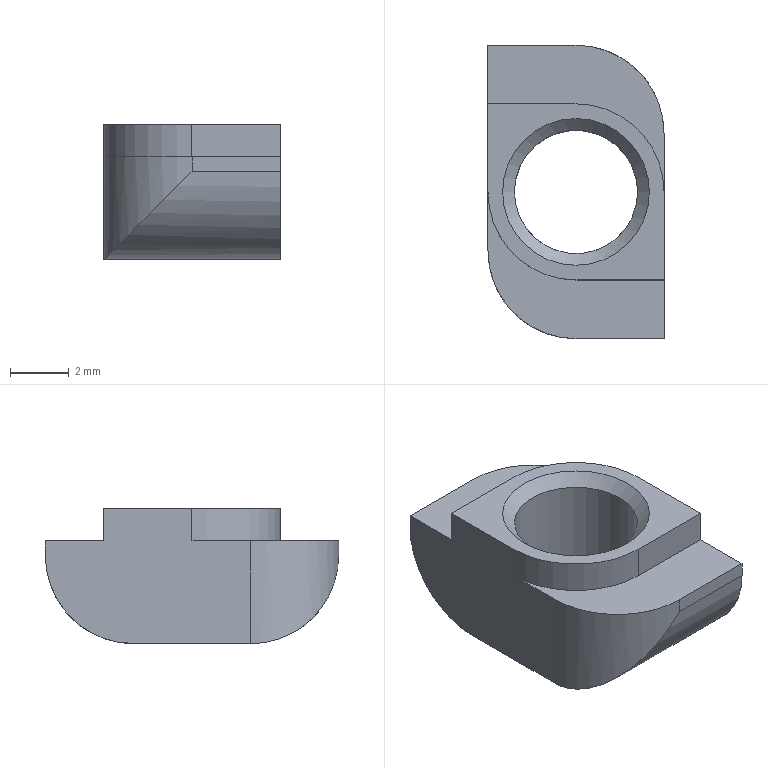Part | NX | features DATUM_CSYS 4, SKETCH 3, EXTRUDE 2, BLEND 1, HOLE PACKAGE 1, SIMPLE HOLE 1, SYMBOLIC_THREAD 1 | 1 solid | 19 faces | box 6 x 10 x 4.6 mm | volume 148.977 mm3 | plane 11 | cylinder 7 | cone 1 | commonest cylinder face diameters 6 x6 4.2 x1
STEP:
#1=CARTESIAN_POINT('',(3.,-2.,-3.5));
#2=VERTEX_POINT('',#1);
#3=CARTESIAN_POINT('',(0.6403,-2.,-3.5));
#4=VERTEX_POINT('',#3);
#5=CARTESIAN_POINT('',(3.,-2.,-3.5));
#6=DIRECTION('',(-1.,0.,0.));
#7=VECTOR('',#6,1000.);
#8=LINE('',#5,#7);
#9=EDGE_CURVE('',#2,#4,#8,.T.);
#10=ORIENTED_EDGE('',*,*,#9,.T.);
#11=CARTESIAN_POINT('',(0.6403,2.,-3.5));
#12=VERTEX_POINT('',#11);
#13=CARTESIAN_POINT('',(0.,0.,-3.5));
#14=DIRECTION('',(0.,0.,1.));
#15=DIRECTION('',(0.,-1.,0.));
#16=AXIS2_PLACEMENT_3D('',#13,#14,#15);
#17=CIRCLE('',#16,2.1);
#18=EDGE_CURVE('',#4,#12,#17,.T.);
#19=ORIENTED_EDGE('',*,*,#18,.T.);
#20=CARTESIAN_POINT('',(3.,2.,-3.5));
#21=VERTEX_POINT('',#20);
#22=CARTESIAN_POINT('',(3.,2.,-3.5));
#23=DIRECTION('',(-1.,0.,0.));
#24=VECTOR('',#23,1000.);
#25=LINE('',#22,#24);
#26=EDGE_CURVE('',#21,#12,#25,.T.);
#27=ORIENTED_EDGE('',*,*,#26,.F.);
#28=CARTESIAN_POINT('',(3.,-2.,-3.5));
#29=DIRECTION('',(0.,1.,0.));
#30=VECTOR('',#29,1000.);
#31=LINE('',#28,#30);
#32=EDGE_CURVE('',#2,#21,#31,.T.);
#33=ORIENTED_EDGE('',*,*,#32,.F.);
#34=EDGE_LOOP('',(#10,#19,#27,#33));
#35=FACE_BOUND('',#34,.T.);
#36=CARTESIAN_POINT('',(3.,0.,-3.5));
#37=DIRECTION('',(0.,0.,1.));
#38=DIRECTION('',(0.,-1.,0.));
#39=AXIS2_PLACEMENT_3D('',#36,#37,#38);
#40=PLANE('',#39);
#41=ADVANCED_FACE('',(#35),#40,.F.);
#42=CARTESIAN_POINT('',(0.,3.,0.));
#43=VERTEX_POINT('',#42);
#44=CARTESIAN_POINT('',(-3.,3.,0.));
#45=VERTEX_POINT('',#44);
#46=CARTESIAN_POINT('',(0.,3.,0.));
#47=DIRECTION('',(-1.,0.,0.));
#48=VECTOR('',#47,1000.);
#49=LINE('',#46,#48);
#50=EDGE_CURVE('',#43,#45,#49,.T.);
#51=ORIENTED_EDGE('',*,*,#50,.F.);
#52=CARTESIAN_POINT('',(3.,0.,0.));
#53=VERTEX_POINT('',#52);
#54=CARTESIAN_POINT('',(0.,0.,0.));
#55=DIRECTION('',(0.,0.,1.));
#56=DIRECTION('',(1.,0.,0.));
#57=AXIS2_PLACEMENT_3D('',#54,#55,#56);
#58=CIRCLE('',#57,3.);
#59=EDGE_CURVE('',#53,#43,#58,.T.);
#60=ORIENTED_EDGE('',*,*,#59,.F.);
#61=CARTESIAN_POINT('',(3.,2.,0.));
#62=VERTEX_POINT('',#61);
#63=CARTESIAN_POINT('',(3.,0.,0.));
#64=DIRECTION('',(0.,-1.,0.));
#65=VECTOR('',#64,1000.);
#66=LINE('',#63,#65);
#67=EDGE_CURVE('',#62,#53,#66,.T.);
#68=ORIENTED_EDGE('',*,*,#67,.F.);
#69=CARTESIAN_POINT('',(0.,5.,0.));
#70=VERTEX_POINT('',#69);
#71=CARTESIAN_POINT('',(0.,2.,0.));
#72=DIRECTION('',(0.,0.,-1.));
#73=DIRECTION('',(-1.,0.,0.));
#74=AXIS2_PLACEMENT_3D('',#71,#72,#73);
#75=CIRCLE('',#74,3.);
#76=EDGE_CURVE('',#62,#70,#75,.F.);
#77=ORIENTED_EDGE('',*,*,#76,.T.);
#78=CARTESIAN_POINT('',(-3.,5.,0.));
#79=VERTEX_POINT('',#78);
#80=CARTESIAN_POINT('',(3.,5.,0.));
#81=DIRECTION('',(-1.,0.,0.));
#82=VECTOR('',#81,1000.);
#83=LINE('',#80,#82);
#84=EDGE_CURVE('',#70,#79,#83,.T.);
#85=ORIENTED_EDGE('',*,*,#84,.T.);
#86=CARTESIAN_POINT('',(-3.,5.,0.));
#87=DIRECTION('',(0.,-1.,0.));
#88=VECTOR('',#87,1000.);
#89=LINE('',#86,#88);
#90=EDGE_CURVE('',#79,#45,#89,.T.);
#91=ORIENTED_EDGE('',*,*,#90,.T.);
#92=EDGE_LOOP('',(#51,#60,#68,#77,#85,#91));
#93=FACE_BOUND('',#92,.T.);
#94=CARTESIAN_POINT('',(3.,5.,0.));
#95=DIRECTION('',(0.,0.,-1.));
#96=DIRECTION('',(-1.,0.,0.));
#97=AXIS2_PLACEMENT_3D('',#94,#95,#96);
#98=PLANE('',#97);
#99=ADVANCED_FACE('',(#93),#98,.F.);
#100=CARTESIAN_POINT('',(3.,-5.,0.));
#101=VERTEX_POINT('',#100);
#102=CARTESIAN_POINT('',(0.,-5.,0.));
#103=VERTEX_POINT('',#102);
#104=CARTESIAN_POINT('',(3.,-5.,0.));
#105=DIRECTION('',(-1.,0.,0.));
#106=VECTOR('',#105,1000.);
#107=LINE('',#104,#106);
#108=EDGE_CURVE('',#101,#103,#107,.T.);
#109=ORIENTED_EDGE('',*,*,#108,.T.);
#110=CARTESIAN_POINT('',(0.,-5.,-0.5));
#111=VERTEX_POINT('',#110);
#112=CARTESIAN_POINT('',(0.,-5.,0.));
#113=DIRECTION('',(0.,0.,-1.));
#114=VECTOR('',#113,1000.);
#115=LINE('',#112,#114);
#116=EDGE_CURVE('',#103,#111,#115,.T.);
#117=ORIENTED_EDGE('',*,*,#116,.T.);
#118=CARTESIAN_POINT('',(3.,-5.,-0.5));
#119=VERTEX_POINT('',#118);
#120=CARTESIAN_POINT('',(3.,-5.,-0.5));
#121=DIRECTION('',(-1.,0.,0.));
#122=VECTOR('',#121,1000.);
#123=LINE('',#120,#122);
#124=EDGE_CURVE('',#119,#111,#123,.T.);
#125=ORIENTED_EDGE('',*,*,#124,.F.);
#126=CARTESIAN_POINT('',(3.,-5.,0.));
#127=DIRECTION('',(0.,0.,-1.));
#128=VECTOR('',#127,1000.);
#129=LINE('',#126,#128);
#130=EDGE_CURVE('',#101,#119,#129,.T.);
#131=ORIENTED_EDGE('',*,*,#130,.F.);
#132=EDGE_LOOP('',(#109,#117,#125,#131));
#133=FACE_BOUND('',#132,.T.);
#134=CARTESIAN_POINT('',(3.,-5.,0.));
#135=DIRECTION('',(0.,1.,0.));
#136=DIRECTION('',(0.,0.,1.));
#137=AXIS2_PLACEMENT_3D('',#134,#135,#136);
#138=PLANE('',#137);
#139=ADVANCED_FACE('',(#133),#138,.F.);
#140=CARTESIAN_POINT('',(-0.6403,-2.,-3.5));
#141=VERTEX_POINT('',#140);
#142=CARTESIAN_POINT('',(-3.,-2.,-3.5));
#143=VERTEX_POINT('',#142);
#144=CARTESIAN_POINT('',(3.,-2.,-3.5));
#145=DIRECTION('',(-1.,0.,0.));
#146=VECTOR('',#145,1000.);
#147=LINE('',#144,#146);
#148=EDGE_CURVE('',#141,#143,#147,.T.);
#149=ORIENTED_EDGE('',*,*,#148,.F.);
#150=CARTESIAN_POINT('',(-0.6403,-2.,-3.5));
#151=CARTESIAN_POINT('',(-0.2238,-2.133,-3.5));
#152=CARTESIAN_POINT('',(0.2238,-2.133,-3.5));
#153=CARTESIAN_POINT('',(0.6403,-2.,-3.5));
#154=B_SPLINE_CURVE_WITH_KNOTS('',3,(#150,#151,#152,#153),.UNSPECIFIED.,.F.,.F.,(4,4),(0.,0.001293),.UNSPECIFIED.);
#155=EDGE_CURVE('',#141,#4,#154,.T.);
#156=ORIENTED_EDGE('',*,*,#155,.T.);
#157=ORIENTED_EDGE('',*,*,#9,.F.);
#158=CARTESIAN_POINT('',(3.,-2.,-0.5));
#159=DIRECTION('',(1.,0.,0.));
#160=DIRECTION('',(0.,1.,0.));
#161=AXIS2_PLACEMENT_3D('',#158,#159,#160);
#162=CIRCLE('',#161,3.);
#163=EDGE_CURVE('',#119,#2,#162,.T.);
#164=ORIENTED_EDGE('',*,*,#163,.F.);
#165=ORIENTED_EDGE('',*,*,#124,.T.);
#166=CARTESIAN_POINT('',(0.,-2.,-0.5));
#167=DIRECTION('',(0.7071,0.,-0.7071));
#168=DIRECTION('',(-0.7071,0.,-0.7071));
#169=AXIS2_PLACEMENT_3D('',#166,#167,#168);
#170=ELLIPSE('',#169,4.243,3.);
#171=EDGE_CURVE('',#111,#143,#170,.T.);
#172=ORIENTED_EDGE('',*,*,#171,.T.);
#173=EDGE_LOOP('',(#149,#156,#157,#164,#165,#172));
#174=FACE_BOUND('',#173,.T.);
#175=CARTESIAN_POINT('',(3.,-2.,-0.5));
#176=DIRECTION('',(-1.,0.,0.));
#177=DIRECTION('',(0.,0.,1.));
#178=AXIS2_PLACEMENT_3D('',#175,#176,#177);
#179=CYLINDRICAL_SURFACE('',#178,3.);
#180=ADVANCED_FACE('',(#174),#179,.T.);
#181=CARTESIAN_POINT('',(-0.6403,2.,-3.5));
#182=VERTEX_POINT('',#181);
#183=CARTESIAN_POINT('',(-3.,2.,-3.5));
#184=VERTEX_POINT('',#183);
#185=CARTESIAN_POINT('',(3.,2.,-3.5));
#186=DIRECTION('',(-1.,0.,0.));
#187=VECTOR('',#186,1000.);
#188=LINE('',#185,#187);
#189=EDGE_CURVE('',#182,#184,#188,.T.);
#190=ORIENTED_EDGE('',*,*,#189,.F.);
#191=CARTESIAN_POINT('',(0.,0.,-3.5));
#192=DIRECTION('',(0.,0.,1.));
#193=DIRECTION('',(0.,-1.,0.));
#194=AXIS2_PLACEMENT_3D('',#191,#192,#193);
#195=CIRCLE('',#194,2.1);
#196=EDGE_CURVE('',#182,#141,#195,.T.);
#197=ORIENTED_EDGE('',*,*,#196,.T.);
#198=ORIENTED_EDGE('',*,*,#148,.T.);
#199=CARTESIAN_POINT('',(-3.,0.,-3.5));
#200=DIRECTION('',(0.,1.,0.));
#201=VECTOR('',#200,1000.);
#202=LINE('',#199,#201);
#203=EDGE_CURVE('',#143,#184,#202,.T.);
#204=ORIENTED_EDGE('',*,*,#203,.T.);
#205=EDGE_LOOP('',(#190,#197,#198,#204));
#206=FACE_BOUND('',#205,.T.);
#207=CARTESIAN_POINT('',(3.,0.,-3.5));
#208=DIRECTION('',(0.,0.,1.));
#209=DIRECTION('',(0.,-1.,0.));
#210=AXIS2_PLACEMENT_3D('',#207,#208,#209);
#211=PLANE('',#210);
#212=ADVANCED_FACE('',(#206),#211,.F.);
#213=ORIENTED_EDGE('',*,*,#26,.T.);
#214=CARTESIAN_POINT('',(0.6403,2.,-3.5));
#215=CARTESIAN_POINT('',(0.2238,2.133,-3.5));
#216=CARTESIAN_POINT('',(-0.2238,2.133,-3.5));
#217=CARTESIAN_POINT('',(-0.6403,2.,-3.5));
#218=B_SPLINE_CURVE_WITH_KNOTS('',3,(#214,#215,#216,#217),.UNSPECIFIED.,.F.,.F.,(4,4),(0.,0.001293),.UNSPECIFIED.);
#219=EDGE_CURVE('',#12,#182,#218,.T.);
#220=ORIENTED_EDGE('',*,*,#219,.T.);
#221=ORIENTED_EDGE('',*,*,#189,.T.);
#222=CARTESIAN_POINT('',(-3.,5.,-0.5));
#223=VERTEX_POINT('',#222);
#224=CARTESIAN_POINT('',(-3.,2.,-0.5));
#225=DIRECTION('',(1.,0.,0.));
#226=DIRECTION('',(0.,-1.,0.));
#227=AXIS2_PLACEMENT_3D('',#224,#225,#226);
#228=CIRCLE('',#227,3.);
#229=EDGE_CURVE('',#184,#223,#228,.T.);
#230=ORIENTED_EDGE('',*,*,#229,.T.);
#231=CARTESIAN_POINT('',(0.,5.,-0.5));
#232=VERTEX_POINT('',#231);
#233=CARTESIAN_POINT('',(3.,5.,-0.5));
#234=DIRECTION('',(-1.,0.,0.));
#235=VECTOR('',#234,1000.);
#236=LINE('',#233,#235);
#237=EDGE_CURVE('',#232,#223,#236,.T.);
#238=ORIENTED_EDGE('',*,*,#237,.F.);
#239=CARTESIAN_POINT('',(0.,2.,-0.5));
#240=DIRECTION('',(-0.7071,0.,-0.7071));
#241=DIRECTION('',(0.7071,0.,-0.7071));
#242=AXIS2_PLACEMENT_3D('',#239,#240,#241);
#243=ELLIPSE('',#242,4.243,3.);
#244=EDGE_CURVE('',#232,#21,#243,.T.);
#245=ORIENTED_EDGE('',*,*,#244,.T.);
#246=EDGE_LOOP('',(#213,#220,#221,#230,#238,#245));
#247=FACE_BOUND('',#246,.T.);
#248=CARTESIAN_POINT('',(3.,2.,-0.5));
#249=DIRECTION('',(-1.,0.,0.));
#250=DIRECTION('',(0.,0.,1.));
#251=AXIS2_PLACEMENT_3D('',#248,#249,#250);
#252=CYLINDRICAL_SURFACE('',#251,3.);
#253=ADVANCED_FACE('',(#247),#252,.T.);
#254=ORIENTED_EDGE('',*,*,#84,.F.);
#255=CARTESIAN_POINT('',(0.,5.,-0.5));
#256=DIRECTION('',(0.,0.,1.));
#257=VECTOR('',#256,1000.);
#258=LINE('',#255,#257);
#259=EDGE_CURVE('',#70,#232,#258,.F.);
#260=ORIENTED_EDGE('',*,*,#259,.T.);
#261=ORIENTED_EDGE('',*,*,#237,.T.);
#262=CARTESIAN_POINT('',(-3.,5.,-0.5));
#263=DIRECTION('',(0.,0.,1.));
#264=VECTOR('',#263,1000.);
#265=LINE('',#262,#264);
#266=EDGE_CURVE('',#223,#79,#265,.T.);
#267=ORIENTED_EDGE('',*,*,#266,.T.);
#268=EDGE_LOOP('',(#254,#260,#261,#267));
#269=FACE_BOUND('',#268,.T.);
#270=CARTESIAN_POINT('',(3.,5.,-0.5));
#271=DIRECTION('',(0.,-1.,0.));
#272=DIRECTION('',(0.,0.,-1.));
#273=AXIS2_PLACEMENT_3D('',#270,#271,#272);
#274=PLANE('',#273);
#275=ADVANCED_FACE('',(#269),#274,.F.);
#276=CARTESIAN_POINT('',(0.,-3.,0.));
#277=VERTEX_POINT('',#276);
#278=CARTESIAN_POINT('',(3.,-3.,0.));
#279=VERTEX_POINT('',#278);
#280=CARTESIAN_POINT('',(0.,-3.,0.));
#281=DIRECTION('',(1.,0.,0.));
#282=VECTOR('',#281,1000.);
#283=LINE('',#280,#282);
#284=EDGE_CURVE('',#277,#279,#283,.T.);
#285=ORIENTED_EDGE('',*,*,#284,.F.);
#286=CARTESIAN_POINT('',(-3.,0.,0.));
#287=VERTEX_POINT('',#286);
#288=CARTESIAN_POINT('',(0.,0.,0.));
#289=DIRECTION('',(0.,0.,1.));
#290=DIRECTION('',(1.,0.,0.));
#291=AXIS2_PLACEMENT_3D('',#288,#289,#290);
#292=CIRCLE('',#291,3.);
#293=EDGE_CURVE('',#287,#277,#292,.T.);
#294=ORIENTED_EDGE('',*,*,#293,.F.);
#295=CARTESIAN_POINT('',(-3.,-2.,0.));
#296=VERTEX_POINT('',#295);
#297=CARTESIAN_POINT('',(-3.,5.,0.));
#298=DIRECTION('',(0.,-1.,0.));
#299=VECTOR('',#298,1000.);
#300=LINE('',#297,#299);
#301=EDGE_CURVE('',#287,#296,#300,.T.);
#302=ORIENTED_EDGE('',*,*,#301,.T.);
#303=CARTESIAN_POINT('',(0.,-2.,0.));
#304=DIRECTION('',(0.,0.,-1.));
#305=DIRECTION('',(-1.,0.,0.));
#306=AXIS2_PLACEMENT_3D('',#303,#304,#305);
#307=CIRCLE('',#306,3.);
#308=EDGE_CURVE('',#296,#103,#307,.F.);
#309=ORIENTED_EDGE('',*,*,#308,.T.);
#310=ORIENTED_EDGE('',*,*,#108,.F.);
#311=CARTESIAN_POINT('',(3.,0.,0.));
#312=DIRECTION('',(0.,-1.,0.));
#313=VECTOR('',#312,1000.);
#314=LINE('',#311,#313);
#315=EDGE_CURVE('',#279,#101,#314,.T.);
#316=ORIENTED_EDGE('',*,*,#315,.F.);
#317=EDGE_LOOP('',(#285,#294,#302,#309,#310,#316));
#318=FACE_BOUND('',#317,.T.);
#319=CARTESIAN_POINT('',(3.,5.,0.));
#320=DIRECTION('',(0.,0.,-1.));
#321=DIRECTION('',(-1.,0.,0.));
#322=AXIS2_PLACEMENT_3D('',#319,#320,#321);
#323=PLANE('',#322);
#324=ADVANCED_FACE('',(#318),#323,.F.);
#325=ORIENTED_EDGE('',*,*,#32,.T.);
#326=CARTESIAN_POINT('',(3.,2.,0.));
#327=DIRECTION('',(0.,0.,1.));
#328=VECTOR('',#327,1000.);
#329=LINE('',#326,#328);
#330=EDGE_CURVE('',#21,#62,#329,.T.);
#331=ORIENTED_EDGE('',*,*,#330,.T.);
#332=ORIENTED_EDGE('',*,*,#67,.T.);
#333=CARTESIAN_POINT('',(3.,0.,1.1));
#334=VERTEX_POINT('',#333);
#335=CARTESIAN_POINT('',(3.,0.,1.1));
#336=DIRECTION('',(0.,0.,-1.));
#337=VECTOR('',#336,1000.);
#338=LINE('',#335,#337);
#339=EDGE_CURVE('',#334,#53,#338,.T.);
#340=ORIENTED_EDGE('',*,*,#339,.F.);
#341=CARTESIAN_POINT('',(3.,-3.,1.1));
#342=VERTEX_POINT('',#341);
#343=CARTESIAN_POINT('',(3.,-3.,1.1));
#344=DIRECTION('',(0.,1.,0.));
#345=VECTOR('',#344,1000.);
#346=LINE('',#343,#345);
#347=EDGE_CURVE('',#342,#334,#346,.T.);
#348=ORIENTED_EDGE('',*,*,#347,.F.);
#349=CARTESIAN_POINT('',(3.,-3.,1.1));
#350=DIRECTION('',(0.,0.,-1.));
#351=VECTOR('',#350,1000.);
#352=LINE('',#349,#351);
#353=EDGE_CURVE('',#342,#279,#352,.T.);
#354=ORIENTED_EDGE('',*,*,#353,.T.);
#355=ORIENTED_EDGE('',*,*,#315,.T.);
#356=ORIENTED_EDGE('',*,*,#130,.T.);
#357=ORIENTED_EDGE('',*,*,#163,.T.);
#358=EDGE_LOOP('',(#325,#331,#332,#340,#348,#354,#355,#356,#357));
#359=FACE_BOUND('',#358,.T.);
#360=CARTESIAN_POINT('',(3.,-2.,-0.5));
#361=DIRECTION('',(1.,0.,0.));
#362=DIRECTION('',(0.,0.,-1.));
#363=AXIS2_PLACEMENT_3D('',#360,#361,#362);
#364=PLANE('',#363);
#365=ADVANCED_FACE('',(#359),#364,.T.);
#366=ORIENTED_EDGE('',*,*,#203,.F.);
#367=CARTESIAN_POINT('',(-3.,-2.,-0.5));
#368=DIRECTION('',(0.,0.,-1.));
#369=VECTOR('',#368,1000.);
#370=LINE('',#367,#369);
#371=EDGE_CURVE('',#143,#296,#370,.F.);
#372=ORIENTED_EDGE('',*,*,#371,.T.);
#373=ORIENTED_EDGE('',*,*,#301,.F.);
#374=CARTESIAN_POINT('',(-3.,0.,1.1));
#375=VERTEX_POINT('',#374);
#376=CARTESIAN_POINT('',(-3.,0.,1.1));
#377=DIRECTION('',(0.,0.,-1.));
#378=VECTOR('',#377,1000.);
#379=LINE('',#376,#378);
#380=EDGE_CURVE('',#375,#287,#379,.T.);
#381=ORIENTED_EDGE('',*,*,#380,.F.);
#382=CARTESIAN_POINT('',(-3.,3.,1.1));
#383=VERTEX_POINT('',#382);
#384=CARTESIAN_POINT('',(-3.,3.,1.1));
#385=DIRECTION('',(0.,-1.,0.));
#386=VECTOR('',#385,1000.);
#387=LINE('',#384,#386);
#388=EDGE_CURVE('',#383,#375,#387,.T.);
#389=ORIENTED_EDGE('',*,*,#388,.F.);
#390=CARTESIAN_POINT('',(-3.,3.,1.1));
#391=DIRECTION('',(0.,0.,-1.));
#392=VECTOR('',#391,1000.);
#393=LINE('',#390,#392);
#394=EDGE_CURVE('',#383,#45,#393,.T.);
#395=ORIENTED_EDGE('',*,*,#394,.T.);
#396=ORIENTED_EDGE('',*,*,#90,.F.);
#397=ORIENTED_EDGE('',*,*,#266,.F.);
#398=ORIENTED_EDGE('',*,*,#229,.F.);
#399=EDGE_LOOP('',(#366,#372,#373,#381,#389,#395,#396,#397,#398));
#400=FACE_BOUND('',#399,.T.);
#401=CARTESIAN_POINT('',(-3.,-2.,-0.5));
#402=DIRECTION('',(1.,0.,0.));
#403=DIRECTION('',(0.,0.,-1.));
#404=AXIS2_PLACEMENT_3D('',#401,#402,#403);
#405=PLANE('',#404);
#406=ADVANCED_FACE('',(#400),#405,.F.);
#407=ORIENTED_EDGE('',*,*,#308,.F.);
#408=ORIENTED_EDGE('',*,*,#371,.F.);
#409=ORIENTED_EDGE('',*,*,#171,.F.);
#410=ORIENTED_EDGE('',*,*,#116,.F.);
#411=EDGE_LOOP('',(#407,#408,#409,#410));
#412=FACE_BOUND('',#411,.T.);
#413=CARTESIAN_POINT('',(0.,-2.,0.));
#414=DIRECTION('',(0.,0.,-1.));
#415=DIRECTION('',(-1.,0.,0.));
#416=AXIS2_PLACEMENT_3D('',#413,#414,#415);
#417=CYLINDRICAL_SURFACE('',#416,3.);
#418=ADVANCED_FACE('',(#412),#417,.T.);
#419=ORIENTED_EDGE('',*,*,#244,.F.);
#420=ORIENTED_EDGE('',*,*,#259,.F.);
#421=ORIENTED_EDGE('',*,*,#76,.F.);
#422=ORIENTED_EDGE('',*,*,#330,.F.);
#423=EDGE_LOOP('',(#419,#420,#421,#422));
#424=FACE_BOUND('',#423,.T.);
#425=CARTESIAN_POINT('',(0.,2.,-0.5));
#426=DIRECTION('',(0.,0.,-1.));
#427=DIRECTION('',(-1.,0.,0.));
#428=AXIS2_PLACEMENT_3D('',#425,#426,#427);
#429=CYLINDRICAL_SURFACE('',#428,3.);
#430=ADVANCED_FACE('',(#424),#429,.T.);
#431=ORIENTED_EDGE('',*,*,#293,.T.);
#432=CARTESIAN_POINT('',(0.,-3.,1.1));
#433=VERTEX_POINT('',#432);
#434=CARTESIAN_POINT('',(0.,-3.,1.1));
#435=DIRECTION('',(0.,0.,-1.));
#436=VECTOR('',#435,1000.);
#437=LINE('',#434,#436);
#438=EDGE_CURVE('',#433,#277,#437,.T.);
#439=ORIENTED_EDGE('',*,*,#438,.F.);
#440=CARTESIAN_POINT('',(0.,0.,1.1));
#441=DIRECTION('',(0.,0.,1.));
#442=DIRECTION('',(1.,0.,0.));
#443=AXIS2_PLACEMENT_3D('',#440,#441,#442);
#444=CIRCLE('',#443,3.);
#445=EDGE_CURVE('',#375,#433,#444,.T.);
#446=ORIENTED_EDGE('',*,*,#445,.F.);
#447=ORIENTED_EDGE('',*,*,#380,.T.);
#448=EDGE_LOOP('',(#431,#439,#446,#447));
#449=FACE_BOUND('',#448,.T.);
#450=CARTESIAN_POINT('',(0.,0.,1.1));
#451=DIRECTION('',(0.,0.,-1.));
#452=DIRECTION('',(-1.,0.,0.));
#453=AXIS2_PLACEMENT_3D('',#450,#451,#452);
#454=CYLINDRICAL_SURFACE('',#453,3.);
#455=ADVANCED_FACE('',(#449),#454,.T.);
#456=ORIENTED_EDGE('',*,*,#284,.T.);
#457=ORIENTED_EDGE('',*,*,#353,.F.);
#458=CARTESIAN_POINT('',(0.,-3.,1.1));
#459=DIRECTION('',(1.,0.,0.));
#460=VECTOR('',#459,1000.);
#461=LINE('',#458,#460);
#462=EDGE_CURVE('',#433,#342,#461,.T.);
#463=ORIENTED_EDGE('',*,*,#462,.F.);
#464=ORIENTED_EDGE('',*,*,#438,.T.);
#465=EDGE_LOOP('',(#456,#457,#463,#464));
#466=FACE_BOUND('',#465,.T.);
#467=CARTESIAN_POINT('',(0.,-3.,1.1));
#468=DIRECTION('',(0.,1.,0.));
#469=DIRECTION('',(-1.,0.,0.));
#470=AXIS2_PLACEMENT_3D('',#467,#468,#469);
#471=PLANE('',#470);
#472=ADVANCED_FACE('',(#466),#471,.F.);
#473=ORIENTED_EDGE('',*,*,#59,.T.);
#474=CARTESIAN_POINT('',(0.,3.,1.1));
#475=VERTEX_POINT('',#474);
#476=CARTESIAN_POINT('',(0.,3.,1.1));
#477=DIRECTION('',(0.,0.,-1.));
#478=VECTOR('',#477,1000.);
#479=LINE('',#476,#478);
#480=EDGE_CURVE('',#475,#43,#479,.T.);
#481=ORIENTED_EDGE('',*,*,#480,.F.);
#482=CARTESIAN_POINT('',(0.,0.,1.1));
#483=DIRECTION('',(0.,0.,1.));
#484=DIRECTION('',(1.,0.,0.));
#485=AXIS2_PLACEMENT_3D('',#482,#483,#484);
#486=CIRCLE('',#485,3.);
#487=EDGE_CURVE('',#334,#475,#486,.T.);
#488=ORIENTED_EDGE('',*,*,#487,.F.);
#489=ORIENTED_EDGE('',*,*,#339,.T.);
#490=EDGE_LOOP('',(#473,#481,#488,#489));
#491=FACE_BOUND('',#490,.T.);
#492=CARTESIAN_POINT('',(0.,0.,1.1));
#493=DIRECTION('',(0.,0.,-1.));
#494=DIRECTION('',(-1.,0.,0.));
#495=AXIS2_PLACEMENT_3D('',#492,#493,#494);
#496=CYLINDRICAL_SURFACE('',#495,3.);
#497=ADVANCED_FACE('',(#491),#496,.T.);
#498=ORIENTED_EDGE('',*,*,#50,.T.);
#499=ORIENTED_EDGE('',*,*,#394,.F.);
#500=CARTESIAN_POINT('',(0.,3.,1.1));
#501=DIRECTION('',(-1.,0.,0.));
#502=VECTOR('',#501,1000.);
#503=LINE('',#500,#502);
#504=EDGE_CURVE('',#475,#383,#503,.T.);
#505=ORIENTED_EDGE('',*,*,#504,.F.);
#506=ORIENTED_EDGE('',*,*,#480,.T.);
#507=EDGE_LOOP('',(#498,#499,#505,#506));
#508=FACE_BOUND('',#507,.T.);
#509=CARTESIAN_POINT('',(0.,3.,1.1));
#510=DIRECTION('',(0.,-1.,0.));
#511=DIRECTION('',(0.,0.,-1.));
#512=AXIS2_PLACEMENT_3D('',#509,#510,#511);
#513=PLANE('',#512);
#514=ADVANCED_FACE('',(#508),#513,.F.);
#515=CARTESIAN_POINT('',(2.5,0.,1.1));
#516=VERTEX_POINT('',#515);
#517=CARTESIAN_POINT('',(0.,0.,1.1));
#518=DIRECTION('',(0.,0.,1.));
#519=DIRECTION('',(1.,0.,0.));
#520=AXIS2_PLACEMENT_3D('',#517,#518,#519);
#521=CIRCLE('',#520,2.5);
#522=EDGE_CURVE('',#516,#516,#521,.F.);
#523=ORIENTED_EDGE('',*,*,#522,.T.);
#524=EDGE_LOOP('',(#523));
#525=FACE_BOUND('',#524,.T.);
#526=ORIENTED_EDGE('',*,*,#388,.T.);
#527=ORIENTED_EDGE('',*,*,#445,.T.);
#528=ORIENTED_EDGE('',*,*,#462,.T.);
#529=ORIENTED_EDGE('',*,*,#347,.T.);
#530=ORIENTED_EDGE('',*,*,#487,.T.);
#531=ORIENTED_EDGE('',*,*,#504,.T.);
#532=EDGE_LOOP('',(#526,#527,#528,#529,#530,#531));
#533=FACE_BOUND('',#532,.T.);
#534=CARTESIAN_POINT('',(0.,0.,1.1));
#535=DIRECTION('',(0.,0.,1.));
#536=DIRECTION('',(1.,0.,0.));
#537=AXIS2_PLACEMENT_3D('',#534,#535,#536);
#538=PLANE('',#537);
#539=ADVANCED_FACE('',(#525,#533),#538,.T.);
#540=CARTESIAN_POINT('',(2.1,0.,0.7));
#541=VERTEX_POINT('',#540);
#542=CARTESIAN_POINT('',(0.,0.,0.7));
#543=DIRECTION('',(0.,0.,1.));
#544=DIRECTION('',(1.,0.,0.));
#545=AXIS2_PLACEMENT_3D('',#542,#543,#544);
#546=CIRCLE('',#545,2.1);
#547=EDGE_CURVE('',#541,#541,#546,.T.);
#548=ORIENTED_EDGE('',*,*,#547,.T.);
#549=EDGE_LOOP('',(#548));
#550=FACE_BOUND('',#549,.T.);
#551=ORIENTED_EDGE('',*,*,#196,.F.);
#552=ORIENTED_EDGE('',*,*,#219,.F.);
#553=ORIENTED_EDGE('',*,*,#18,.F.);
#554=ORIENTED_EDGE('',*,*,#155,.F.);
#555=EDGE_LOOP('',(#551,#552,#553,#554));
#556=FACE_BOUND('',#555,.T.);
#557=CARTESIAN_POINT('',(0.,0.,1.1));
#558=DIRECTION('',(0.,0.,-1.));
#559=DIRECTION('',(-1.,0.,0.));
#560=AXIS2_PLACEMENT_3D('',#557,#558,#559);
#561=CYLINDRICAL_SURFACE('',#560,2.1);
#562=ADVANCED_FACE('',(#550,#556),#561,.F.);
#563=ORIENTED_EDGE('',*,*,#547,.F.);
#564=EDGE_LOOP('',(#563));
#565=FACE_BOUND('',#564,.T.);
#566=ORIENTED_EDGE('',*,*,#522,.F.);
#567=EDGE_LOOP('',(#566));
#568=FACE_BOUND('',#567,.T.);
#569=CARTESIAN_POINT('',(0.,0.,1.1));
#570=DIRECTION('',(0.,0.,1.));
#571=DIRECTION('',(1.,0.,0.));
#572=AXIS2_PLACEMENT_3D('',#569,#570,#571);
#573=CONICAL_SURFACE('',#572,2.5,0.7854);
#574=ADVANCED_FACE('',(#565,#568),#573,.F.);
#575=CLOSED_SHELL('',(#41,#99,#139,#180,#212,#253,#275,#324,#365,#406,#418,#430,#455,#472,#497,#514,#539,#562,#574));
#576=MANIFOLD_SOLID_BREP('',#575);
#577=(LENGTH_UNIT()NAMED_UNIT(*)SI_UNIT(.MILLI.,.METRE.));
#578=UNCERTAINTY_MEASURE_WITH_UNIT(LENGTH_MEASURE(0.0508),#577,'','');
#579=(NAMED_UNIT(*)PLANE_ANGLE_UNIT()SI_UNIT($,.RADIAN.));
#580=(NAMED_UNIT(*)SI_UNIT($,.STERADIAN.)SOLID_ANGLE_UNIT());
#581=(GEOMETRIC_REPRESENTATION_CONTEXT(3)GLOBAL_UNCERTAINTY_ASSIGNED_CONTEXT((#578))GLOBAL_UNIT_ASSIGNED_CONTEXT((#577,#579,#580))REPRESENTATION_CONTEXT('',''));
#582=ADVANCED_BREP_SHAPE_REPRESENTATION('',(#576),#581);